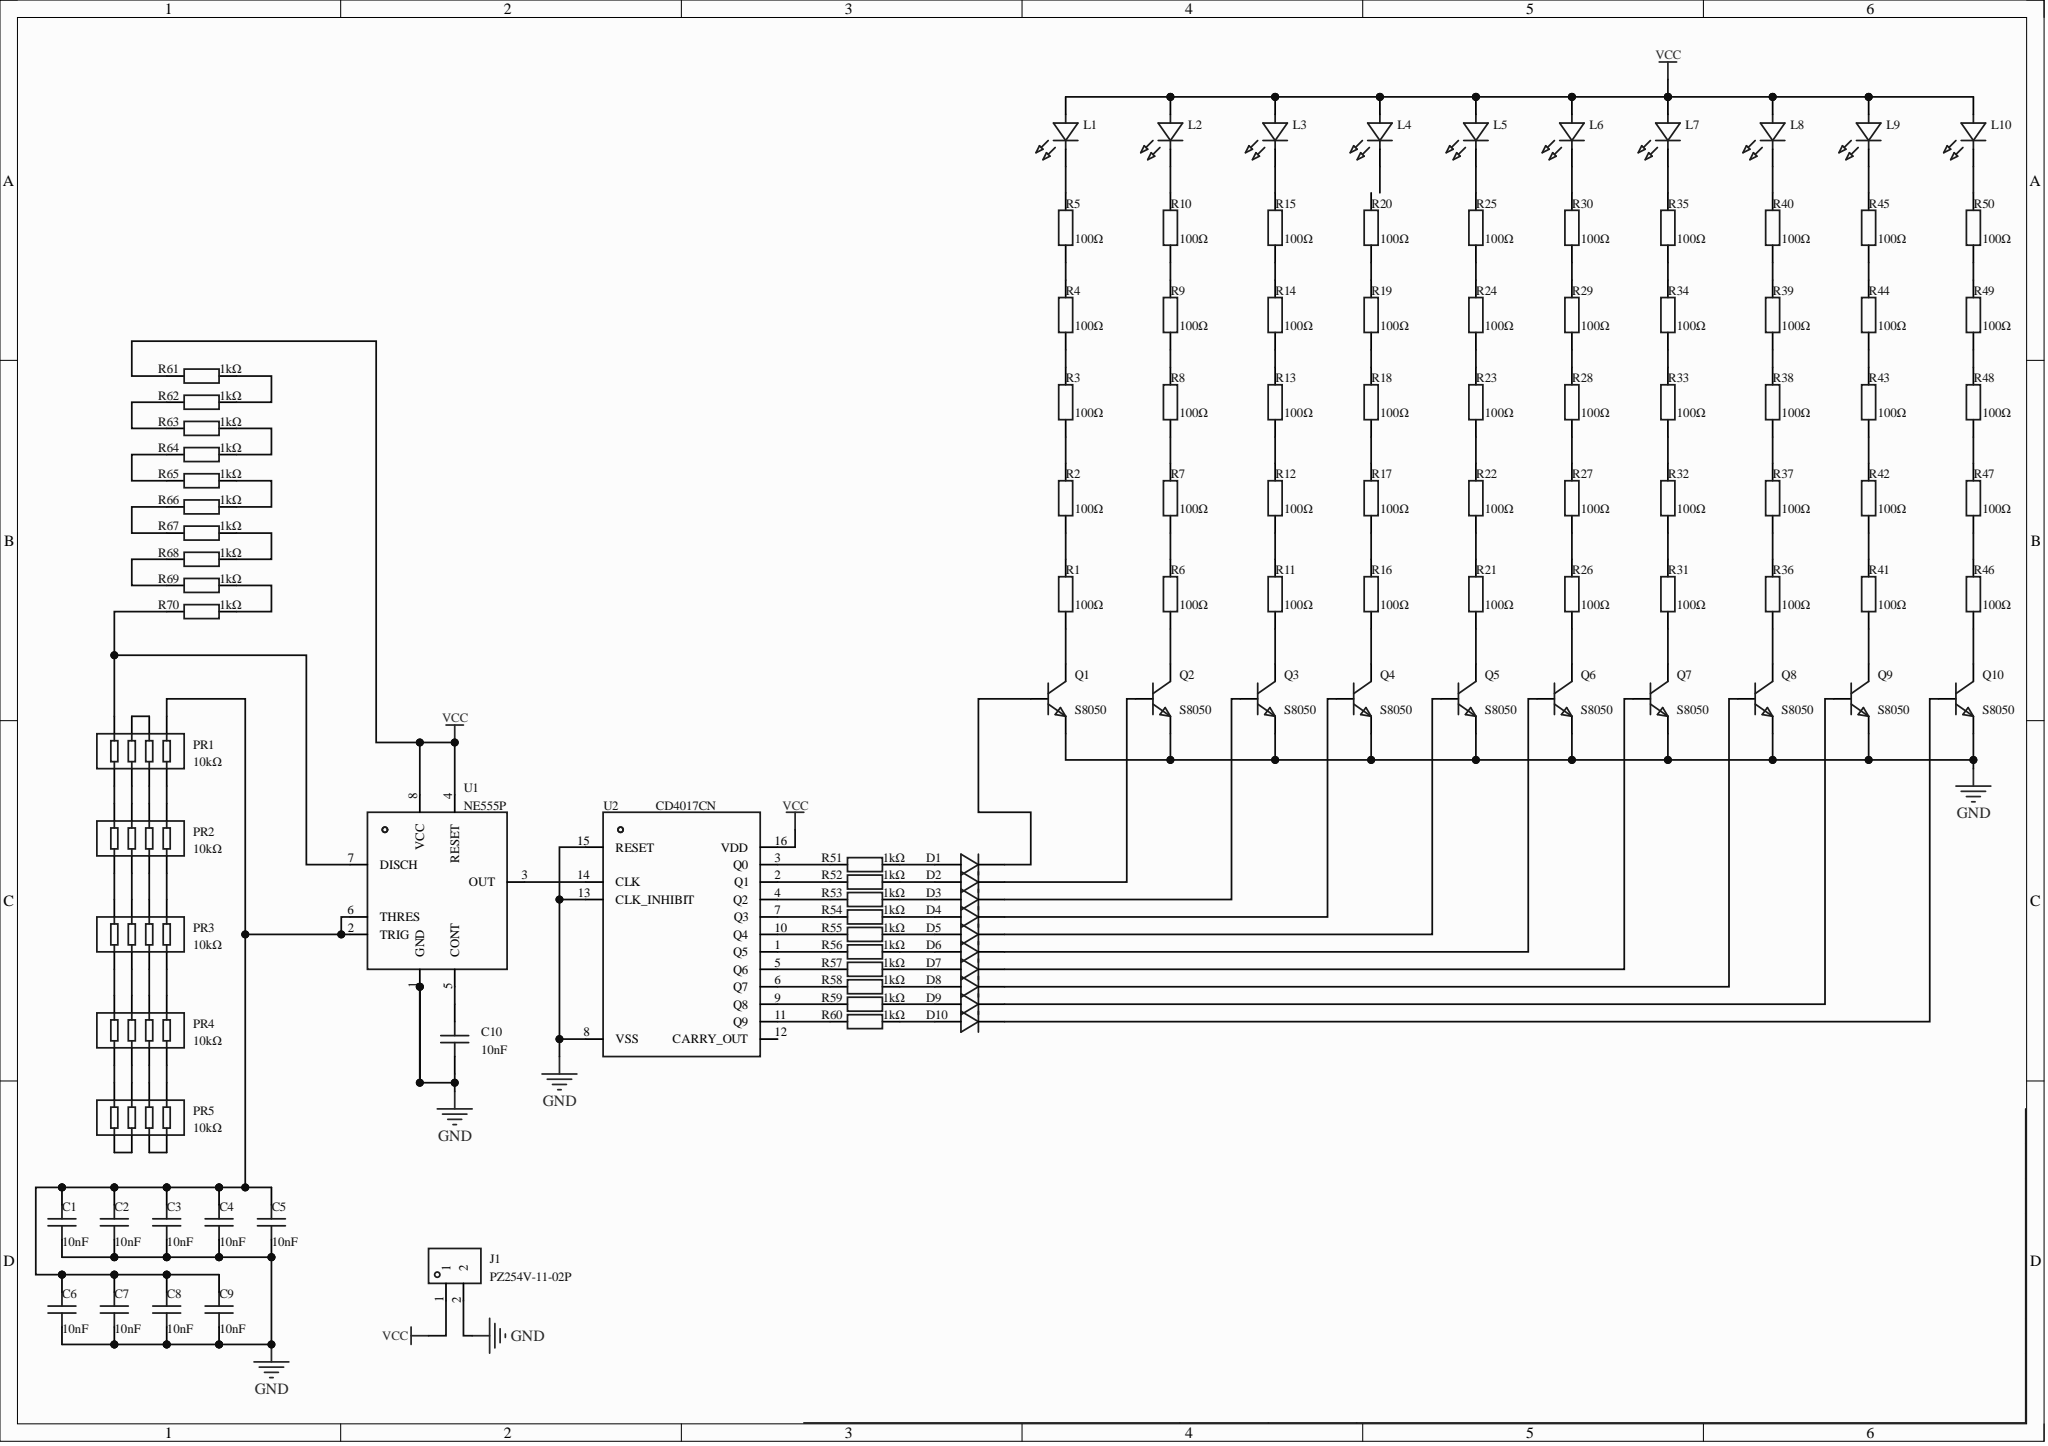Circuit board | Altium Designer | 118 parts | 123 nets
Bill of materials:
Comment,Description,Designator,Footprint,LibRef,Quantity
"10nF","容值:10nF;精度:±20%;额定电压:1kV;温度系数:Y5V;","C1, C2, C3, C4, C5, C6, C7, C8, C9, C10","CAP-TH_L8.0-W2.8-P5.08-D0.6","CC3A103MC1IEF48C30MF","10"
"1N4148TR","二极管配置:-;正向压降(Vf):1V@10mA;直流反向耐压(Vr):100V;整流电流:200mA;反向恢复时间(Trr):4ns;","D1, D2, D3, D4, D5, D6, D7, D8, D9, D10","DO-35_BD2.0-L4.2-P8.20-D0.5-RD","1N4148TR_C84410","10"
"PZ254V-11-02P","插针结构:1x2P;间距:2.54mm;行距:-;圆针/方针:方针;安装方式:直插;排数:单排;总PIN位数:2P;额定电流:3A;额定电压:250V;配合针长度:6mm;塑高:2.5mm;端接针长度:3mm;触头材质:黄铜;触头镀层:-;工作温度:-40℃~+105℃;颜色:黑色;","J1","HDR-TH_2P-P2.54-V-M","PZ254V-11-02P","1"
"XL-502SURD","灯头类型:5mm圆形灯头;发光颜色:红色;正向压降(Vf):2.4V;功率:70mW;正向电流:20mA;波长:615nm~625nm;二极管配置:-;透镜颜色:红色透镜;色温:-;发光强度:300mcd;发光角度:35°;载带方式:-;工作温度:-25℃~+85℃;","L1, L2, L3, L4, L5, L6, L7, L8, L9, L10","LED-TH_BD5.9-P2.54-RD_RED","XL-502SURD","10"
"10kΩ","","PR1, PR2, PR3, PR4, PR5","RES-ARRAY-TH_8P-L20.3-W2.5-P2.54","4608X-102-103LF","5"
"S8050","晶体管类型:NPN;集电极电流(Ic):500mA;集射极击穿电压(Vceo):25V;耗散功率(Pd):625mW;直流电流增益(hFE):160@50mA,1V;","Q1, Q2, Q3, Q4, Q5, Q6, Q7, Q8, Q9, Q10","TO-92-3_L4.5-W3.5-P1.27-L","S8050_C2931492","10"
"100Ω","","R1, R2, R3, R4, R5, R6, R7, R8, R9, R10, R11, R12, R13, R14, R15, R16, R17, R18, R19, R20, R21, R22, R23, R24, R25, R26, R27, R28, R29, R30, R31, R32, R33, R34, R35, R36, R37, R38, R39, R40, R41, R42, R43, R44, R45, R46, R47, R48, R49, R50","RES-TH_BD2.2-L6.5-P10.50-D0.6","MFR0W4F1000A50","50"
"1kΩ","","R51, R52, R53, R54, R55, R56, R57, R58, R59, R60, R61, R62, R63, R64, R65, R66, R67, R68, R69, R70","RES-TH_BD2.5-L6.5-P10.50-D0.6","MFR0W4F1001A50","20"
"NE555P","这些器件是精密定时电路，能够产生精确的时间延迟或振荡。在延时或单稳态工作模式下，定时时间间隔由单个外部电阻和电容网络控制。在无稳态工作模式下，频率和占空比可通过两个外部电阻和一个外部电容分别控制","U1","DIP-8_L9.8-W6.6-P2.54-LS7.6-BL","NE555P","1"
"CD4017CN","CD4017BE升级替代料，建议试样，5 阶 Johnson 译码计数器","U2","PDIP-16_L19.3-W6.4-P2.54-LS7.94-BL","CD4017CN","1"
Netlist (Protel format):
[
C1
CAP-TH_L8.0-W2.8-P5.08-D0.6
10nF



]
[
C2
CAP-TH_L8.0-W2.8-P5.08-D0.6
10nF



]
[
C3
CAP-TH_L8.0-W2.8-P5.08-D0.6
10nF



]
[
C4
CAP-TH_L8.0-W2.8-P5.08-D0.6
10nF



]
[
C5
CAP-TH_L8.0-W2.8-P5.08-D0.6
10nF



]
[
C6
CAP-TH_L8.0-W2.8-P5.08-D0.6
10nF



]
[
C7
CAP-TH_L8.0-W2.8-P5.08-D0.6
10nF



]
[
C8
CAP-TH_L8.0-W2.8-P5.08-D0.6
10nF



]
[
C9
CAP-TH_L8.0-W2.8-P5.08-D0.6
10nF



]
[
C10
CAP-TH_L8.0-W2.8-P5.08-D0.6
10nF



]
[
D1
DO-35_BD2.0-L4.2-P8.20-D0.5-RD
1N4148TR



]
[
D2
DO-35_BD2.0-L4.2-P8.20-D0.5-RD
1N4148TR



]
[
D3
DO-35_BD2.0-L4.2-P8.20-D0.5-RD
1N4148TR



]
[
D4
DO-35_BD2.0-L4.2-P8.20-D0.5-RD
1N4148TR



]
[
D5
DO-35_BD2.0-L4.2-P8.20-D0.5-RD
1N4148TR



]
[
D6
DO-35_BD2.0-L4.2-P8.20-D0.5-RD
1N4148TR



]
[
D7
DO-35_BD2.0-L4.2-P8.20-D0.5-RD
1N4148TR



]
[
D8
DO-35_BD2.0-L4.2-P8.20-D0.5-RD
1N4148TR



]
[
D9
DO-35_BD2.0-L4.2-P8.20-D0.5-RD
1N4148TR



]
[
D10
DO-35_BD2.0-L4.2-P8.20-D0.5-RD
1N4148TR



]
[
J1
HDR-TH_2P-P2.54-V-M
PZ254V-11-02P



]
[
L1
LED-TH_BD5.9-P2.54-RD_RED
XL-502SURD



]
[
L2
LED-TH_BD5.9-P2.54-RD_RED
XL-502SURD



]
[
L3
LED-TH_BD5.9-P2.54-RD_RED
XL-502SURD



]
[
L4
LED-TH_BD5.9-P2.54-RD_RED
XL-502SURD



]
[
L5
LED-TH_BD5.9-P2.54-RD_RED
XL-502SURD



]
[
L6
LED-TH_BD5.9-P2.54-RD_RED
XL-502SURD



]
[
L7
LED-TH_BD5.9-P2.54-RD_RED
XL-502SURD



]
[
L8
LED-TH_BD5.9-P2.54-RD_RED
XL-502SURD



]
[
L9
LED-TH_BD5.9-P2.54-RD_RED
XL-502SURD



]
[
L10
LED-TH_BD5.9-P2.54-RD_RED
XL-502SURD



]
[
PR1
RES-ARRAY-TH_8P-L20.3-W2.5-P2.54
10kΩ



]
[
PR2
RES-ARRAY-TH_8P-L20.3-W2.5-P2.54
10kΩ



]
[
PR3
RES-ARRAY-TH_8P-L20.3-W2.5-P2.54
10kΩ



]
[
PR4
RES-ARRAY-TH_8P-L20.3-W2.5-P2.54
10kΩ



]
[
PR5
RES-ARRAY-TH_8P-L20.3-W2.5-P2.54
10kΩ



]
[
Q1
TO-92-3_L4.5-W3.5-P1.27-L
S8050



]
[
Q2
TO-92-3_L4.5-W3.5-P1.27-L
S8050



]
[
Q3
TO-92-3_L4.5-W3.5-P1.27-L
S8050



]
[
Q4
TO-92-3_L4.5-W3.5-P1.27-L
S8050



]
[
Q5
TO-92-3_L4.5-W3.5-P1.27-L
S8050



]
[
Q6
TO-92-3_L4.5-W3.5-P1.27-L
S8050



]
[
Q7
TO-92-3_L4.5-W3.5-P1.27-L
S8050



]
[
Q8
TO-92-3_L4.5-W3.5-P1.27-L
S8050



]
[
Q9
TO-92-3_L4.5-W3.5-P1.27-L
S8050



]
[
Q10
TO-92-3_L4.5-W3.5-P1.27-L
S8050



]
[
R1
RES-TH_BD2.2-L6.5-P10.50-D0.6
100Ω



]
[
R2
RES-TH_BD2.2-L6.5-P10.50-D0.6
100Ω



]
[
R3
RES-TH_BD2.2-L6.5-P10.50-D0.6
100Ω



]
[
R4
RES-TH_BD2.2-L6.5-P10.50-D0.6
100Ω



]
[
R5
RES-TH_BD2.2-L6.5-P10.50-D0.6
100Ω



]
[
R6
RES-TH_BD2.2-L6.5-P10.50-D0.6
100Ω



]
[
R7
RES-TH_BD2.2-L6.5-P10.50-D0.6
100Ω



]
[
R8
RES-TH_BD2.2-L6.5-P10.50-D0.6
100Ω



]
[
R9
RES-TH_BD2.2-L6.5-P10.50-D0.6
100Ω



]
[
R10
RES-TH_BD2.2-L6.5-P10.50-D0.6
100Ω



]
[
R11
RES-TH_BD2.2-L6.5-P10.50-D0.6
100Ω



]
[
R12
RES-TH_BD2.2-L6.5-P10.50-D0.6
100Ω



]
[
R13
RES-TH_BD2.2-L6.5-P10.50-D0.6
100Ω



]
[
R14
RES-TH_BD2.2-L6.5-P10.50-D0.6
100Ω



]
[
R15
RES-TH_BD2.2-L6.5-P10.50-D0.6
100Ω



]
[
R16
RES-TH_BD2.2-L6.5-P10.50-D0.6
100Ω



]
[
R17
RES-TH_BD2.2-L6.5-P10.50-D0.6
100Ω



]
[
R18
RES-TH_BD2.2-L6.5-P10.50-D0.6
100Ω



]
[
R19
RES-TH_BD2.2-L6.5-P10.50-D0.6
100Ω



]
[
R20
RES-TH_BD2.2-L6.5-P10.50-D0.6
100Ω



]
[
R21
RES-TH_BD2.2-L6.5-P10.50-D0.6
100Ω



]
[
R22
RES-TH_BD2.2-L6.5-P10.50-D0.6
100Ω



]
[
R23
RES-TH_BD2.2-L6.5-P10.50-D0.6
100Ω



]
[
R24
RES-TH_BD2.2-L6.5-P10.50-D0.6
100Ω



]
[
R25
RES-TH_BD2.2-L6.5-P10.50-D0.6
100Ω



]
[
R26
RES-TH_BD2.2-L6.5-P10.50-D0.6
100Ω



]
[
R27
RES-TH_BD2.2-L6.5-P10.50-D0.6
100Ω



]
[
R28
RES-TH_BD2.2-L6.5-P10.50-D0.6
100Ω



]
[
R29
RES-TH_BD2.2-L6.5-P10.50-D0.6
100Ω



]
[
R30
RES-TH_BD2.2-L6.5-P10.50-D0.6
100Ω



]
[
R31
RES-TH_BD2.2-L6.5-P10.50-D0.6
100Ω



]
[
R32
RES-TH_BD2.2-L6.5-P10.50-D0.6
100Ω



]
[
R33
RES-TH_BD2.2-L6.5-P10.50-D0.6
100Ω



]
[
R34
RES-TH_BD2.2-L6.5-P10.50-D0.6
100Ω



]
[
R35
RES-TH_BD2.2-L6.5-P10.50-D0.6
100Ω



]
[
R36
RES-TH_BD2.2-L6.5-P10.50-D0.6
100Ω



]
[
R37
RES-TH_BD2.2-L6.5-P10.50-D0.6
100Ω



]
[
R38
RES-TH_BD2.2-L6.5-P10.50-D0.6
100Ω



]
[
R39
RES-TH_BD2.2-L6.5-P10.50-D0.6
100Ω



]
[
R40
RES-TH_BD2.2-L6.5-P10.50-D0.6
100Ω



]
[
R41
RES-TH_BD2.2-L6.5-P10.50-D0.6
100Ω



]
[
R42
RES-TH_BD2.2-L6.5-P10.50-D0.6
100Ω



]
[
R43
RES-TH_BD2.2-L6.5-P10.50-D0.6
100Ω



]
[
R44
RES-TH_BD2.2-L6.5-P10.50-D0.6
100Ω



]
[
R45
RES-TH_BD2.2-L6.5-P10.50-D0.6
100Ω



]
[
R46
RES-TH_BD2.2-L6.5-P10.50-D0.6
100Ω



]
[
R47
RES-TH_BD2.2-L6.5-P10.50-D0.6
100Ω



]
[
R48
RES-TH_BD2.2-L6.5-P10.50-D0.6
100Ω



]
[
R49
RES-TH_BD2.2-L6.5-P10.50-D0.6
100Ω



]
[
R50
RES-TH_BD2.2-L6.5-P10.50-D0.6
100Ω



]
[
R51
RES-TH_BD2.5-L6.5-P10.50-D0.6
1kΩ



]
[
R52
RES-TH_BD2.5-L6.5-P10.50-D0.6
1kΩ



]
[
R53
RES-TH_BD2.5-L6.5-P10.50-D0.6
1kΩ



]
[
R54
RES-TH_BD2.5-L6.5-P10.50-D0.6
1kΩ



]
[
R55
RES-TH_BD2.5-L6.5-P10.50-D0.6
1kΩ



]
[
R56
RES-TH_BD2.5-L6.5-P10.50-D0.6
1kΩ



]
[
R57
RES-TH_BD2.5-L6.5-P10.50-D0.6
1kΩ



]
[
R58
RES-TH_BD2.5-L6.5-P10.50-D0.6
1kΩ



]
[
R59
RES-TH_BD2.5-L6.5-P10.50-D0.6
1kΩ



]
[
R60
RES-TH_BD2.5-L6.5-P10.50-D0.6
1kΩ



]
[
R61
RES-TH_BD2.5-L6.5-P10.50-D0.6
1kΩ



]
[
R62
RES-TH_BD2.5-L6.5-P10.50-D0.6
1kΩ



]
[
R63
RES-TH_BD2.5-L6.5-P10.50-D0.6
1kΩ



]
[
R64
RES-TH_BD2.5-L6.5-P10.50-D0.6
1kΩ



]
[
R65
RES-TH_BD2.5-L6.5-P10.50-D0.6
1kΩ



]
[
R66
RES-TH_BD2.5-L6.5-P10.50-D0.6
1kΩ



]
[
R67
RES-TH_BD2.5-L6.5-P10.50-D0.6
1kΩ



]
[
R68
RES-TH_BD2.5-L6.5-P10.50-D0.6
1kΩ



]
[
R69
RES-TH_BD2.5-L6.5-P10.50-D0.6
1kΩ



]
[
R70
RES-TH_BD2.5-L6.5-P10.50-D0.6
1kΩ



]
[
U1
DIP-8_L9.8-W6.6-P2.54-LS7.6-BL
NE555P



]
[
U2
PDIP-16_L19.3-W6.4-P2.54-LS7.94-BL
CD4017CN



]
(
VCC
J1-1
L1-2
L2-2
L3-2
L4-2
L5-2
L6-2
L7-2
L8-2
L9-2
L10-2
R61-1
U1-4
U1-8
U2-16
)
(
NetU1_3
U1-3
U2-14
)
(
NetR69_2
R69-2
R70-2
)
(
NetR68_1
R68-1
R69-1
)
(
NetR67_2
R67-2
R68-2
)
(
NetR66_1
R66-1
R67-1
)
(
NetR65_2
R65-2
R66-2
)
(
NetR64_1
R64-1
R65-1
)
(
NetR63_2
R63-2
R64-2
)
(
NetR62_1
R62-1
R63-1
)
(
NetR61_2
R61-2
R62-2
)
(
NetR60_1
R60-1
U2-11
)
(
NetR59_1
R59-1
U2-9
)
(
NetR58_1
R58-1
U2-6
)
(
NetR57_1
R57-1
U2-5
)
(
NetR56_1
R56-1
U2-1
)
(
NetR55_1
R55-1
U2-10
)
(
NetR54_1
R54-1
U2-7
)
(
NetR53_1
R53-1
U2-4
)
(
NetR52_1
R52-1
U2-2
)
(
NetR51_1
R51-1
U2-3
)
(
NetR49_2
R49-2
R50-1
)
(
NetR48_2
R48-2
R49-1
)
(
NetR47_2
R47-2
R48-1
)
(
NetR46_2
R46-2
R47-1
)
(
NetR44_2
R44-2
R45-1
)
(
NetR43_2
R43-2
R44-1
)
(
NetR42_2
R42-2
R43-1
)
(
NetR41_2
R41-2
R42-1
)
(
NetR39_2
R39-2
R40-1
)
(
NetR38_2
R38-2
R39-1
)
(
NetR37_2
R37-2
R38-1
)
(
NetR36_2
R36-2
R37-1
)
(
NetR34_2
R34-2
R35-1
)
(
NetR33_2
R33-2
R34-1
)
(
NetR32_2
R32-2
R33-1
)
(
NetR31_2
R31-2
R32-1
)
(
NetR29_2
R29-2
R30-1
)
(
NetR28_2
R28-2
R29-1
)
(
NetR27_2
R27-2
R28-1
)
(
NetR26_2
R26-2
R27-1
)
(
NetR24_2
R24-2
R25-1
)
(
NetR23_2
R23-2
R24-1
)
(
NetR22_2
R22-2
R23-1
)
(
NetR21_2
R21-2
R22-1
)
(
NetR19_2
R19-2
R20-1
)
(
NetR18_2
R18-2
R19-1
)
(
NetR17_2
R17-2
R18-1
)
(
NetR16_2
R16-2
R17-1
)
(
NetR14_2
R14-2
R15-1
)
(
NetR13_2
R13-2
R14-1
)
(
NetR12_2
R12-2
R13-1
)
(
NetR11_2
R11-2
R12-1
)
(
NetR9_2
R9-2
R10-1
)
(
NetR8_2
R8-2
R9-1
)
(
NetR7_2
R7-2
R8-1
)
(
NetR6_2
R6-2
R7-1
)
(
NetR4_2
R4-2
R5-1
)
(
NetR3_2
R3-2
R4-1
)
(
NetR2_2
R2-2
R3-1
)
(
NetR1_2
R1-2
R2-1
)
(
NetQ10_3
Q10-3
R46-1
)
(
NetQ9_3
Q9-3
R41-1
)
(
NetQ8_3
Q8-3
R36-1
)
(
NetQ7_3
Q7-3
R31-1
)
(
NetQ6_3
Q6-3
R26-1
)
(
NetQ5_3
Q5-3
R21-1
)
(
NetQ4_3
Q4-3
R16-1
)
(
NetQ3_3
Q3-3
R11-1
)
(
NetQ2_3
Q2-3
R6-1
)
(
NetQ1_3
Q1-3
R1-1
)
(
NetPR5_3
PR5-3
PR5-4
)
(
NetPR5_1
PR5-1
PR5-2
)
(
NetPR4_4
PR4-4
PR5-5
)
(
NetPR4_3
PR4-3
PR5-6
)
(
NetPR4_2
PR4-2
PR5-7
)
(
NetPR4_1
PR4-1
PR5-8
)
(
NetPR3_4
PR3-4
PR4-5
)
(
NetPR3_3
PR3-3
PR4-6
)
(
NetPR3_2
PR3-2
PR4-7
)
(
NetPR3_1
PR3-1
PR4-8
)
(
NetPR2_4
PR2-4
PR3-5
)
(
NetPR2_3
PR2-3
PR3-6
)
(
NetPR2_2
PR2-2
PR3-7
)
(
NetPR2_1
PR2-1
PR3-8
)
(
NetPR1_8
PR1-8
R70-1
U1-7
)
(
NetPR1_6
PR1-6
PR1-7
)
(
NetPR1_4
PR1-4
PR2-5
)
(
NetPR1_3
PR1-3
PR2-6
)
(
NetPR1_2
PR1-2
PR2-7
)
(
NetPR1_1
PR1-1
PR2-8
)
(
NetL10_1
L10-1
R50-2
)
(
NetL9_1
L9-1
R45-2
)
(
NetL8_1
L8-1
R40-2
)
(
NetL7_1
L7-1
R35-2
)
(
NetL6_1
L6-1
R30-2
)
(
NetL5_1
L5-1
R25-2
)
(
NetL3_1
L3-1
R15-2
)
(
NetL2_1
L2-1
R10-2
)
(
NetL1_1
L1-1
R5-2
)
(
NetD10_2
D10-2
R60-2
)
(
NetD10_1
D10-1
Q10-2
)
(
NetD9_2
D9-2
R59-2
)
(
NetD9_1
D9-1
Q9-2
)
(
NetD8_2
D8-2
R58-2
)
(
NetD8_1
D8-1
Q8-2
)
(
NetD7_2
D7-2
R57-2
)
(
NetD7_1
D7-1
Q7-2
)
(
NetD6_2
D6-2
R56-2
)
(
NetD6_1
D6-1
Q6-2
)
(
NetD5_2
D5-2
R55-2
)
(
NetD5_1
D5-1
Q5-2
)
(
NetD4_2
D4-2
R54-2
)
(
NetD4_1
D4-1
Q4-2
)
(
NetD3_2
D3-2
R53-2
)
(
NetD3_1
D3-1
Q3-2
)
(
NetD2_2
D2-2
R52-2
)
(
NetD2_1
D2-1
Q2-2
)
(
NetD1_2
D1-2
R51-2
)
(
NetD1_1
D1-1
Q1-2
)
(
NetC10_2
C10-2
U1-5
)
(
NetC1_2
C1-2
C2-2
C3-2
C4-2
C5-2
C6-2
C7-2
C8-2
C9-2
PR1-5
U1-2
U1-6
)
(
GND
C1-1
C2-1
C3-1
C4-1
C5-1
C6-1
C7-1
C8-1
C9-1
C10-1
J1-2
Q1-1
Q2-1
Q3-1
Q4-1
Q5-1
Q6-1
Q7-1
Q8-1
Q9-1
Q10-1
U1-1
U2-8
U2-13
U2-15
)